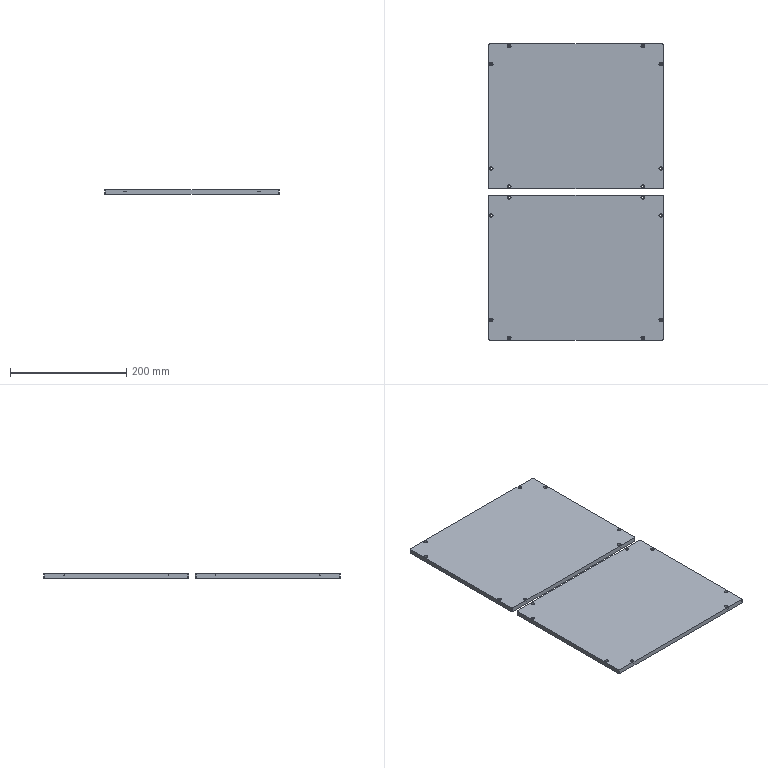CAM job | NX | 3-axis milling | part box 300 x 511 x 8 mm | stock box 304 x 515 x 8 mm
Tools:
number,name,description,diameter,corner_radius,flute_length,length,flutes
2,D4A45,Milling Tool-5 Parameters,4.0,0.0,2.0,2.0,2
4,D4,Milling Tool-5 Parameters,4.0,0.0,50.0,75.0,2
12,D2,Milling Tool-5 Parameters,2.0,0.0,50.0,75.0,2
10,D10JING,Milling Tool-5 Parameters,10.0,0.0,50.0,75.0,2
Operations:
program,operation,operation_type,tool,method,geometry_group,spindle_rpm,surface_speed,feed_per_tooth,feed_cut,feed_plunge,cut_length_mm,path_length_mm,cut_time_min,machine_time_min
1,ZLEVEL_PROFILE_1_COPY_1_COPY,ZLevelMilling,D4A45,METHOD,A,9500.0,179.0,0.0526,1000.0,100.0,2504.081,8706.045,2.504,3.124
1,HOLE_MILLING,CylinderMilling,D4,METHOD,A,9500.0,179.0,0.0658,1250.0,100.0,1492.736,3839.461,1.194,1.429
1,HOLE_MILLING_COPY,CylinderMilling,D2,METHOD,A,9500.0,59.0,0.0579,1100.0,100.0,2552.208,5024.533,2.32,2.567
1,ZLEVEL_PROFILE,ZLevelMilling,D10JING,METHOD,A,9500.0,298.0,0.0789,1500.0,1000.0,18271.823,18922.598,12.213,12.278